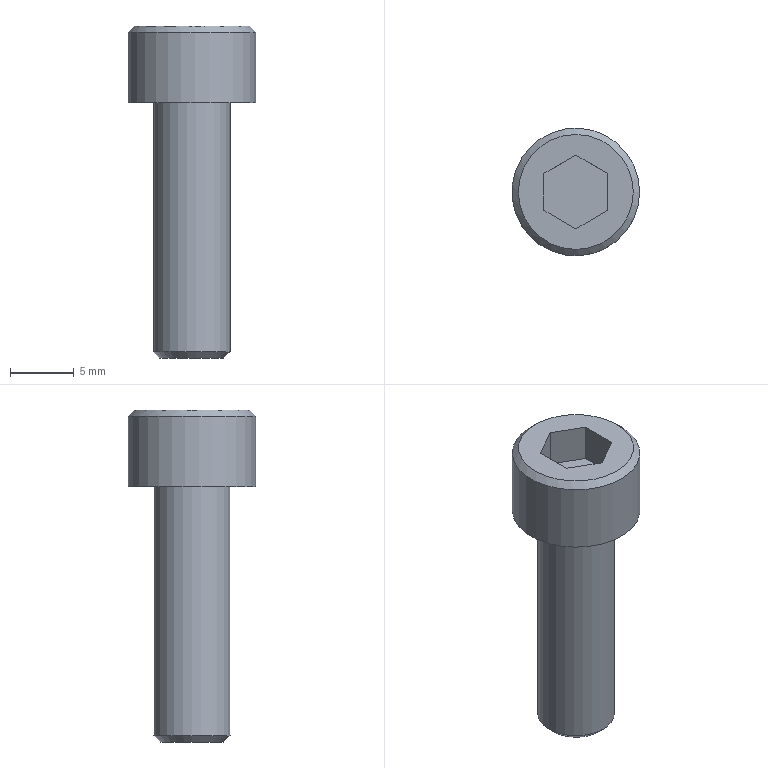Part | STEP file | M6.00-20.00 | 1 solid | 14 faces | box 10 x 10 x 26 mm | volume 965.752 mm3 | plane 10 | cylinder 2 | cone 2 | commonest cylinder face diameters 6 x1 10 x1